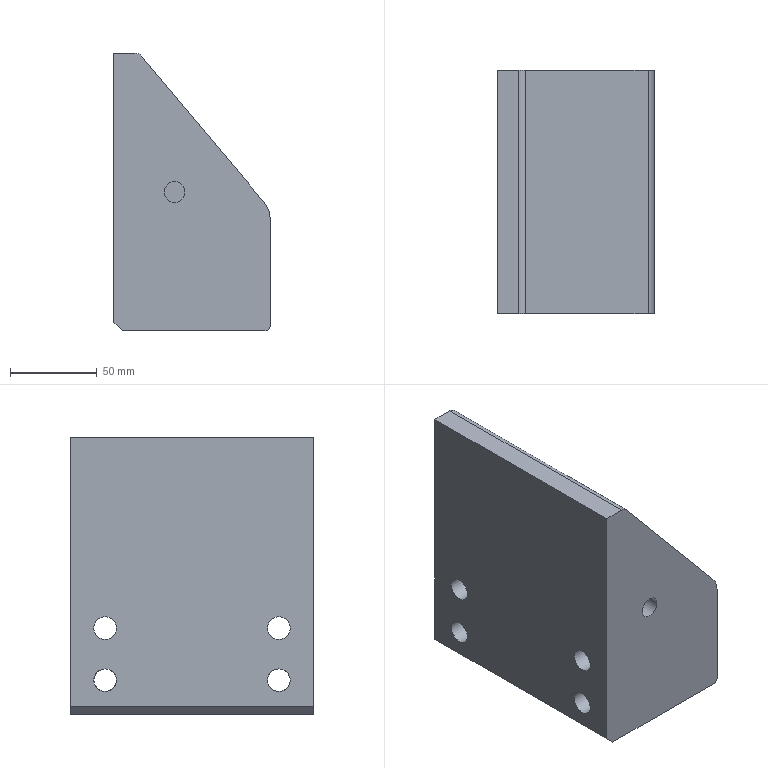Part | NX | features MAIN_BODY 2 | 1 solid | 27 faces | box 90 x 140 x 160 mm | volume 1435895 mm3 | plane 14 | cylinder 13 | commonest cylinder face diameters 13 x4 20 x4 12 x2 6 x1 10 x1 30 x1
STEP:
#1=CARTESIAN_POINT('',(780.,255.,-157.));
#2=VERTEX_POINT('',#1);
#3=CARTESIAN_POINT('',(780.,255.,-95.46));
#4=VERTEX_POINT('',#3);
#5=CARTESIAN_POINT('',(780.,255.,34.907));
#6=DIRECTION('',(0.,0.,1.));
#7=VECTOR('',#6,1000.);
#8=LINE('',#5,#7);
#9=EDGE_CURVE('',#2,#4,#8,.T.);
#10=ORIENTED_EDGE('',*,*,#9,.T.);
#11=CARTESIAN_POINT('',(780.,115.,-95.46));
#12=VERTEX_POINT('',#11);
#13=CARTESIAN_POINT('',(780.,145.,-95.46));
#14=DIRECTION('',(0.,1.,0.));
#15=VECTOR('',#14,1000.);
#16=LINE('',#13,#15);
#17=EDGE_CURVE('',#4,#12,#16,.F.);
#18=ORIENTED_EDGE('',*,*,#17,.T.);
#19=CARTESIAN_POINT('',(780.,115.,-157.));
#20=VERTEX_POINT('',#19);
#21=CARTESIAN_POINT('',(780.,115.,-165.));
#22=DIRECTION('',(0.,0.,-1.));
#23=VECTOR('',#22,1000.);
#24=LINE('',#21,#23);
#25=EDGE_CURVE('',#12,#20,#24,.T.);
#26=ORIENTED_EDGE('',*,*,#25,.T.);
#27=CARTESIAN_POINT('',(780.,350.,-157.));
#28=DIRECTION('',(0.,1.,0.));
#29=VECTOR('',#28,1000.);
#30=LINE('',#27,#29);
#31=EDGE_CURVE('',#20,#2,#30,.T.);
#32=ORIENTED_EDGE('',*,*,#31,.T.);
#33=EDGE_LOOP('',(#10,#18,#26,#32));
#34=FACE_BOUND('',#33,.T.);
#35=CARTESIAN_POINT('',(780.,135.,-100.));
#36=VERTEX_POINT('',#35);
#37=CARTESIAN_POINT('',(780.,135.,-110.));
#38=DIRECTION('',(1.,0.,0.));
#39=DIRECTION('',(0.,0.,1.));
#40=AXIS2_PLACEMENT_3D('',#37,#38,#39);
#41=CIRCLE('',#40,10.);
#42=EDGE_CURVE('',#36,#36,#41,.T.);
#43=ORIENTED_EDGE('',*,*,#42,.F.);
#44=EDGE_LOOP('',(#43));
#45=FACE_BOUND('',#44,.T.);
#46=CARTESIAN_POINT('',(780.,245.,-140.));
#47=VERTEX_POINT('',#46);
#48=CARTESIAN_POINT('',(780.,235.,-140.));
#49=DIRECTION('',(1.,0.,0.));
#50=DIRECTION('',(0.,1.,0.));
#51=AXIS2_PLACEMENT_3D('',#48,#49,#50);
#52=CIRCLE('',#51,10.);
#53=EDGE_CURVE('',#47,#47,#52,.F.);
#54=ORIENTED_EDGE('',*,*,#53,.T.);
#55=EDGE_LOOP('',(#54));
#56=FACE_BOUND('',#55,.T.);
#57=CARTESIAN_POINT('',(780.,235.,-100.));
#58=VERTEX_POINT('',#57);
#59=CARTESIAN_POINT('',(780.,235.,-110.));
#60=DIRECTION('',(1.,0.,0.));
#61=DIRECTION('',(0.,0.,1.));
#62=AXIS2_PLACEMENT_3D('',#59,#60,#61);
#63=CIRCLE('',#62,10.);
#64=EDGE_CURVE('',#58,#58,#63,.T.);
#65=ORIENTED_EDGE('',*,*,#64,.F.);
#66=EDGE_LOOP('',(#65));
#67=FACE_BOUND('',#66,.T.);
#68=CARTESIAN_POINT('',(780.,145.,-140.));
#69=VERTEX_POINT('',#68);
#70=CARTESIAN_POINT('',(780.,135.,-140.));
#71=DIRECTION('',(1.,0.,0.));
#72=DIRECTION('',(0.,1.,0.));
#73=AXIS2_PLACEMENT_3D('',#70,#71,#72);
#74=CIRCLE('',#73,10.);
#75=EDGE_CURVE('',#69,#69,#74,.F.);
#76=ORIENTED_EDGE('',*,*,#75,.T.);
#77=EDGE_LOOP('',(#76));
#78=FACE_BOUND('',#77,.T.);
#79=CARTESIAN_POINT('',(780.,350.,-165.));
#80=DIRECTION('',(1.,0.,0.));
#81=DIRECTION('',(0.,1.,0.));
#82=AXIS2_PLACEMENT_3D('',#79,#80,#81);
#83=PLANE('',#82);
#84=ADVANCED_FACE('',(#34,#45,#56,#67,#78),#83,.T.);
#85=CARTESIAN_POINT('',(725.,255.,-74.));
#86=VERTEX_POINT('',#85);
#87=CARTESIAN_POINT('',(725.,255.,-80.));
#88=DIRECTION('',(0.,-1.,0.));
#89=DIRECTION('',(0.,0.,1.));
#90=AXIS2_PLACEMENT_3D('',#87,#88,#89);
#91=CIRCLE('',#90,6.);
#92=EDGE_CURVE('',#86,#86,#91,.T.);
#93=ORIENTED_EDGE('',*,*,#92,.F.);
#94=EDGE_LOOP('',(#93));
#95=FACE_BOUND('',#94,.T.);
#96=CARTESIAN_POINT('',(725.,225.,-74.));
#97=VERTEX_POINT('',#96);
#98=CARTESIAN_POINT('',(725.,225.,-80.));
#99=DIRECTION('',(0.,-1.,0.));
#100=DIRECTION('',(0.,0.,1.));
#101=AXIS2_PLACEMENT_3D('',#98,#99,#100);
#102=CIRCLE('',#101,6.);
#103=EDGE_CURVE('',#97,#97,#102,.F.);
#104=ORIENTED_EDGE('',*,*,#103,.F.);
#105=EDGE_LOOP('',(#104));
#106=FACE_BOUND('',#105,.T.);
#107=CARTESIAN_POINT('',(725.,320.,-80.));
#108=DIRECTION('',(0.,1.,0.));
#109=DIRECTION('',(0.,0.,-1.));
#110=AXIS2_PLACEMENT_3D('',#107,#108,#109);
#111=CYLINDRICAL_SURFACE('',#110,6.);
#112=ADVANCED_FACE('',(#95,#106),#111,.F.);
#113=CARTESIAN_POINT('',(776.491,115.,-85.818));
#114=VERTEX_POINT('',#113);
#115=CARTESIAN_POINT('',(705.98,115.,-1.786));
#116=VERTEX_POINT('',#115);
#117=CARTESIAN_POINT('',(780.,115.,-90.));
#118=DIRECTION('',(-0.6428,0.,0.766));
#119=VECTOR('',#118,1000.);
#120=LINE('',#117,#119);
#121=EDGE_CURVE('',#114,#116,#120,.T.);
#122=ORIENTED_EDGE('',*,*,#121,.F.);
#123=CARTESIAN_POINT('',(776.491,255.,-85.818));
#124=VERTEX_POINT('',#123);
#125=CARTESIAN_POINT('',(776.491,275.,-85.818));
#126=DIRECTION('',(0.,1.,0.));
#127=VECTOR('',#126,1000.);
#128=LINE('',#125,#127);
#129=EDGE_CURVE('',#114,#124,#128,.T.);
#130=ORIENTED_EDGE('',*,*,#129,.T.);
#131=CARTESIAN_POINT('',(705.98,255.,-1.786));
#132=VERTEX_POINT('',#131);
#133=CARTESIAN_POINT('',(780.,255.,-90.));
#134=DIRECTION('',(-0.6428,0.,0.766));
#135=VECTOR('',#134,1000.);
#136=LINE('',#133,#135);
#137=EDGE_CURVE('',#124,#132,#136,.T.);
#138=ORIENTED_EDGE('',*,*,#137,.T.);
#139=CARTESIAN_POINT('',(705.98,175.,-1.786));
#140=DIRECTION('',(0.,1.,0.));
#141=VECTOR('',#140,1000.);
#142=LINE('',#139,#141);
#143=EDGE_CURVE('',#132,#116,#142,.F.);
#144=ORIENTED_EDGE('',*,*,#143,.T.);
#145=EDGE_LOOP('',(#122,#130,#138,#144));
#146=FACE_BOUND('',#145,.T.);
#147=CARTESIAN_POINT('',(780.,225.,-90.));
#148=DIRECTION('',(-0.766,0.,-0.6428));
#149=DIRECTION('',(0.6428,0.,-0.766));
#150=AXIS2_PLACEMENT_3D('',#147,#148,#149);
#151=PLANE('',#150);
#152=ADVANCED_FACE('',(#146),#151,.F.);
#153=CARTESIAN_POINT('',(690.,235.,-103.5));
#154=VERTEX_POINT('',#153);
#155=CARTESIAN_POINT('',(690.,235.,-110.));
#156=DIRECTION('',(1.,0.,0.));
#157=DIRECTION('',(0.,0.,1.));
#158=AXIS2_PLACEMENT_3D('',#155,#156,#157);
#159=CIRCLE('',#158,6.5);
#160=EDGE_CURVE('',#154,#154,#159,.F.);
#161=ORIENTED_EDGE('',*,*,#160,.T.);
#162=EDGE_LOOP('',(#161));
#163=FACE_BOUND('',#162,.T.);
#164=CARTESIAN_POINT('',(715.,235.,-103.5));
#165=VERTEX_POINT('',#164);
#166=CARTESIAN_POINT('',(715.,235.,-110.));
#167=DIRECTION('',(1.,0.,0.));
#168=DIRECTION('',(0.,0.,1.));
#169=AXIS2_PLACEMENT_3D('',#166,#167,#168);
#170=CIRCLE('',#169,6.5);
#171=EDGE_CURVE('',#165,#165,#170,.T.);
#172=ORIENTED_EDGE('',*,*,#171,.T.);
#173=EDGE_LOOP('',(#172));
#174=FACE_BOUND('',#173,.T.);
#175=CARTESIAN_POINT('',(780.,235.,-110.));
#176=DIRECTION('',(-1.,0.,0.));
#177=DIRECTION('',(0.,0.,-1.));
#178=AXIS2_PLACEMENT_3D('',#175,#176,#177);
#179=CYLINDRICAL_SURFACE('',#178,6.5);
#180=ADVANCED_FACE('',(#163,#174),#179,.F.);
#181=CARTESIAN_POINT('',(690.,135.,-103.5));
#182=VERTEX_POINT('',#181);
#183=CARTESIAN_POINT('',(690.,135.,-110.));
#184=DIRECTION('',(1.,0.,0.));
#185=DIRECTION('',(0.,0.,1.));
#186=AXIS2_PLACEMENT_3D('',#183,#184,#185);
#187=CIRCLE('',#186,6.5);
#188=EDGE_CURVE('',#182,#182,#187,.F.);
#189=ORIENTED_EDGE('',*,*,#188,.T.);
#190=EDGE_LOOP('',(#189));
#191=FACE_BOUND('',#190,.T.);
#192=CARTESIAN_POINT('',(715.,135.,-103.5));
#193=VERTEX_POINT('',#192);
#194=CARTESIAN_POINT('',(715.,135.,-110.));
#195=DIRECTION('',(1.,0.,0.));
#196=DIRECTION('',(0.,0.,1.));
#197=AXIS2_PLACEMENT_3D('',#194,#195,#196);
#198=CIRCLE('',#197,6.5);
#199=EDGE_CURVE('',#193,#193,#198,.T.);
#200=ORIENTED_EDGE('',*,*,#199,.T.);
#201=EDGE_LOOP('',(#200));
#202=FACE_BOUND('',#201,.T.);
#203=CARTESIAN_POINT('',(780.,135.,-110.));
#204=DIRECTION('',(-1.,0.,0.));
#205=DIRECTION('',(0.,0.,-1.));
#206=AXIS2_PLACEMENT_3D('',#203,#204,#205);
#207=CYLINDRICAL_SURFACE('',#206,6.5);
#208=ADVANCED_FACE('',(#191,#202),#207,.F.);
#209=CARTESIAN_POINT('',(690.,135.,-133.5));
#210=VERTEX_POINT('',#209);
#211=CARTESIAN_POINT('',(690.,135.,-140.));
#212=DIRECTION('',(-1.,0.,0.));
#213=DIRECTION('',(0.,0.,1.));
#214=AXIS2_PLACEMENT_3D('',#211,#212,#213);
#215=CIRCLE('',#214,6.5);
#216=EDGE_CURVE('',#210,#210,#215,.T.);
#217=ORIENTED_EDGE('',*,*,#216,.F.);
#218=EDGE_LOOP('',(#217));
#219=FACE_BOUND('',#218,.T.);
#220=CARTESIAN_POINT('',(690.,235.,-133.5));
#221=VERTEX_POINT('',#220);
#222=CARTESIAN_POINT('',(690.,235.,-140.));
#223=DIRECTION('',(-1.,0.,0.));
#224=DIRECTION('',(0.,0.,1.));
#225=AXIS2_PLACEMENT_3D('',#222,#223,#224);
#226=CIRCLE('',#225,6.5);
#227=EDGE_CURVE('',#221,#221,#226,.T.);
#228=ORIENTED_EDGE('',*,*,#227,.F.);
#229=EDGE_LOOP('',(#228));
#230=FACE_BOUND('',#229,.T.);
#231=ORIENTED_EDGE('',*,*,#160,.F.);
#232=EDGE_LOOP('',(#231));
#233=FACE_BOUND('',#232,.T.);
#234=CARTESIAN_POINT('',(690.,255.,-155.));
#235=VERTEX_POINT('',#234);
#236=CARTESIAN_POINT('',(690.,255.,0.));
#237=VERTEX_POINT('',#236);
#238=CARTESIAN_POINT('',(690.,255.,34.907));
#239=DIRECTION('',(0.,0.,1.));
#240=VECTOR('',#239,1000.);
#241=LINE('',#238,#240);
#242=EDGE_CURVE('',#235,#237,#241,.T.);
#243=ORIENTED_EDGE('',*,*,#242,.F.);
#244=CARTESIAN_POINT('',(690.,115.,-155.));
#245=VERTEX_POINT('',#244);
#246=CARTESIAN_POINT('',(690.,175.,-155.));
#247=DIRECTION('',(0.,-1.,0.));
#248=VECTOR('',#247,1000.);
#249=LINE('',#246,#248);
#250=EDGE_CURVE('',#235,#245,#249,.T.);
#251=ORIENTED_EDGE('',*,*,#250,.T.);
#252=CARTESIAN_POINT('',(690.,115.,0.));
#253=VERTEX_POINT('',#252);
#254=CARTESIAN_POINT('',(690.,115.,-165.));
#255=DIRECTION('',(0.,0.,-1.));
#256=VECTOR('',#255,1000.);
#257=LINE('',#254,#256);
#258=EDGE_CURVE('',#253,#245,#257,.T.);
#259=ORIENTED_EDGE('',*,*,#258,.F.);
#260=CARTESIAN_POINT('',(690.,255.,0.));
#261=DIRECTION('',(0.,1.,0.));
#262=VECTOR('',#261,1000.);
#263=LINE('',#260,#262);
#264=EDGE_CURVE('',#253,#237,#263,.T.);
#265=ORIENTED_EDGE('',*,*,#264,.T.);
#266=EDGE_LOOP('',(#243,#251,#259,#265));
#267=FACE_BOUND('',#266,.T.);
#268=ORIENTED_EDGE('',*,*,#188,.F.);
#269=EDGE_LOOP('',(#268));
#270=FACE_BOUND('',#269,.T.);
#271=CARTESIAN_POINT('',(690.,350.,-165.));
#272=DIRECTION('',(1.,0.,0.));
#273=DIRECTION('',(0.,1.,0.));
#274=AXIS2_PLACEMENT_3D('',#271,#272,#273);
#275=PLANE('',#274);
#276=ADVANCED_FACE('',(#219,#230,#233,#267,#270),#275,.F.);
#277=CARTESIAN_POINT('',(702.149,115.,0.));
#278=VERTEX_POINT('',#277);
#279=CARTESIAN_POINT('',(780.078,115.,0.));
#280=DIRECTION('',(-1.,0.,0.));
#281=VECTOR('',#280,1000.);
#282=LINE('',#279,#281);
#283=EDGE_CURVE('',#278,#253,#282,.T.);
#284=ORIENTED_EDGE('',*,*,#283,.F.);
#285=CARTESIAN_POINT('',(702.149,255.,0.));
#286=VERTEX_POINT('',#285);
#287=CARTESIAN_POINT('',(702.149,325.,0.));
#288=DIRECTION('',(0.,1.,0.));
#289=VECTOR('',#288,1000.);
#290=LINE('',#287,#289);
#291=EDGE_CURVE('',#278,#286,#290,.T.);
#292=ORIENTED_EDGE('',*,*,#291,.T.);
#293=CARTESIAN_POINT('',(780.078,255.,0.));
#294=DIRECTION('',(-1.,0.,0.));
#295=VECTOR('',#294,1000.);
#296=LINE('',#293,#295);
#297=EDGE_CURVE('',#286,#237,#296,.T.);
#298=ORIENTED_EDGE('',*,*,#297,.T.);
#299=ORIENTED_EDGE('',*,*,#264,.F.);
#300=EDGE_LOOP('',(#284,#292,#298,#299));
#301=FACE_BOUND('',#300,.T.);
#302=CARTESIAN_POINT('',(400.,255.,0.));
#303=DIRECTION('',(0.,0.,1.));
#304=DIRECTION('',(-1.,0.,0.));
#305=AXIS2_PLACEMENT_3D('',#302,#303,#304);
#306=PLANE('',#305);
#307=ADVANCED_FACE('',(#301),#306,.T.);
#308=CARTESIAN_POINT('',(777.,115.,-160.));
#309=VERTEX_POINT('',#308);
#310=CARTESIAN_POINT('',(695.,115.,-160.));
#311=VERTEX_POINT('',#310);
#312=CARTESIAN_POINT('',(720.,115.,-160.));
#313=DIRECTION('',(-1.,0.,0.));
#314=VECTOR('',#313,1000.);
#315=LINE('',#312,#314);
#316=EDGE_CURVE('',#309,#311,#315,.T.);
#317=ORIENTED_EDGE('',*,*,#316,.T.);
#318=CARTESIAN_POINT('',(695.,255.,-160.));
#319=VERTEX_POINT('',#318);
#320=CARTESIAN_POINT('',(695.,325.,-160.));
#321=DIRECTION('',(0.,1.,0.));
#322=VECTOR('',#321,1000.);
#323=LINE('',#320,#322);
#324=EDGE_CURVE('',#311,#319,#323,.T.);
#325=ORIENTED_EDGE('',*,*,#324,.T.);
#326=CARTESIAN_POINT('',(777.,255.,-160.));
#327=VERTEX_POINT('',#326);
#328=CARTESIAN_POINT('',(780.078,255.,-160.));
#329=DIRECTION('',(1.,0.,0.));
#330=VECTOR('',#329,1000.);
#331=LINE('',#328,#330);
#332=EDGE_CURVE('',#319,#327,#331,.T.);
#333=ORIENTED_EDGE('',*,*,#332,.T.);
#334=CARTESIAN_POINT('',(777.,350.,-160.));
#335=DIRECTION('',(0.,1.,0.));
#336=VECTOR('',#335,1000.);
#337=LINE('',#334,#336);
#338=EDGE_CURVE('',#327,#309,#337,.F.);
#339=ORIENTED_EDGE('',*,*,#338,.T.);
#340=EDGE_LOOP('',(#317,#325,#333,#339));
#341=FACE_BOUND('',#340,.T.);
#342=CARTESIAN_POINT('',(720.,350.,-160.));
#343=DIRECTION('',(0.,0.,-1.));
#344=DIRECTION('',(0.,1.,0.));
#345=AXIS2_PLACEMENT_3D('',#342,#343,#344);
#346=PLANE('',#345);
#347=ADVANCED_FACE('',(#341),#346,.T.);
#348=CARTESIAN_POINT('',(725.,115.,-74.));
#349=VERTEX_POINT('',#348);
#350=CARTESIAN_POINT('',(725.,115.,-80.));
#351=DIRECTION('',(0.,-1.,0.));
#352=DIRECTION('',(0.,0.,1.));
#353=AXIS2_PLACEMENT_3D('',#350,#351,#352);
#354=CIRCLE('',#353,6.);
#355=EDGE_CURVE('',#349,#349,#354,.T.);
#356=ORIENTED_EDGE('',*,*,#355,.F.);
#357=EDGE_LOOP('',(#356));
#358=FACE_BOUND('',#357,.T.);
#359=ORIENTED_EDGE('',*,*,#25,.F.);
#360=CARTESIAN_POINT('',(765.,115.,-95.46));
#361=DIRECTION('',(0.,-1.,0.));
#362=DIRECTION('',(0.,0.,1.));
#363=AXIS2_PLACEMENT_3D('',#360,#361,#362);
#364=CIRCLE('',#363,15.);
#365=EDGE_CURVE('',#12,#114,#364,.T.);
#366=ORIENTED_EDGE('',*,*,#365,.T.);
#367=ORIENTED_EDGE('',*,*,#121,.T.);
#368=CARTESIAN_POINT('',(702.149,115.,-5.));
#369=DIRECTION('',(0.,-1.,0.));
#370=DIRECTION('',(0.,0.,1.));
#371=AXIS2_PLACEMENT_3D('',#368,#369,#370);
#372=CIRCLE('',#371,5.);
#373=EDGE_CURVE('',#116,#278,#372,.T.);
#374=ORIENTED_EDGE('',*,*,#373,.T.);
#375=ORIENTED_EDGE('',*,*,#283,.T.);
#376=ORIENTED_EDGE('',*,*,#258,.T.);
#377=CARTESIAN_POINT('',(632.586,115.,-97.586));
#378=DIRECTION('',(0.7071,0.,-0.7071));
#379=VECTOR('',#378,1000.);
#380=LINE('',#377,#379);
#381=EDGE_CURVE('',#245,#311,#380,.T.);
#382=ORIENTED_EDGE('',*,*,#381,.T.);
#383=ORIENTED_EDGE('',*,*,#316,.F.);
#384=CARTESIAN_POINT('',(777.,115.,-157.));
#385=DIRECTION('',(0.,-1.,0.));
#386=DIRECTION('',(0.,0.,1.));
#387=AXIS2_PLACEMENT_3D('',#384,#385,#386);
#388=CIRCLE('',#387,3.);
#389=EDGE_CURVE('',#309,#20,#388,.T.);
#390=ORIENTED_EDGE('',*,*,#389,.T.);
#391=EDGE_LOOP('',(#359,#366,#367,#374,#375,#376,#382,#383,#390));
#392=FACE_BOUND('',#391,.T.);
#393=CARTESIAN_POINT('',(780.078,115.,34.907));
#394=DIRECTION('',(0.,-1.,0.));
#395=DIRECTION('',(0.,0.,-1.));
#396=AXIS2_PLACEMENT_3D('',#393,#394,#395);
#397=PLANE('',#396);
#398=ADVANCED_FACE('',(#358,#392),#397,.T.);
#399=ORIENTED_EDGE('',*,*,#92,.T.);
#400=EDGE_LOOP('',(#399));
#401=FACE_BOUND('',#400,.T.);
#402=ORIENTED_EDGE('',*,*,#137,.F.);
#403=CARTESIAN_POINT('',(765.,255.,-95.46));
#404=DIRECTION('',(0.,-1.,0.));
#405=DIRECTION('',(0.,0.,1.));
#406=AXIS2_PLACEMENT_3D('',#403,#404,#405);
#407=CIRCLE('',#406,15.);
#408=EDGE_CURVE('',#124,#4,#407,.F.);
#409=ORIENTED_EDGE('',*,*,#408,.T.);
#410=ORIENTED_EDGE('',*,*,#9,.F.);
#411=CARTESIAN_POINT('',(777.,255.,-157.));
#412=DIRECTION('',(0.,-1.,0.));
#413=DIRECTION('',(0.,0.,1.));
#414=AXIS2_PLACEMENT_3D('',#411,#412,#413);
#415=CIRCLE('',#414,3.);
#416=EDGE_CURVE('',#2,#327,#415,.F.);
#417=ORIENTED_EDGE('',*,*,#416,.T.);
#418=ORIENTED_EDGE('',*,*,#332,.F.);
#419=CARTESIAN_POINT('',(695.,255.,-160.));
#420=DIRECTION('',(-0.7071,0.,0.7071));
#421=VECTOR('',#420,1000.);
#422=LINE('',#419,#421);
#423=EDGE_CURVE('',#319,#235,#422,.T.);
#424=ORIENTED_EDGE('',*,*,#423,.T.);
#425=ORIENTED_EDGE('',*,*,#242,.T.);
#426=ORIENTED_EDGE('',*,*,#297,.F.);
#427=CARTESIAN_POINT('',(702.149,255.,-5.));
#428=DIRECTION('',(0.,-1.,0.));
#429=DIRECTION('',(0.,0.,1.));
#430=AXIS2_PLACEMENT_3D('',#427,#428,#429);
#431=CIRCLE('',#430,5.);
#432=EDGE_CURVE('',#286,#132,#431,.F.);
#433=ORIENTED_EDGE('',*,*,#432,.T.);
#434=EDGE_LOOP('',(#402,#409,#410,#417,#418,#424,#425,#426,#433));
#435=FACE_BOUND('',#434,.T.);
#436=CARTESIAN_POINT('',(780.078,255.,34.907));
#437=DIRECTION('',(0.,-1.,0.));
#438=DIRECTION('',(0.,0.,-1.));
#439=AXIS2_PLACEMENT_3D('',#436,#437,#438);
#440=PLANE('',#439);
#441=ADVANCED_FACE('',(#401,#435),#440,.F.);
#442=ORIENTED_EDGE('',*,*,#42,.T.);
#443=EDGE_LOOP('',(#442));
#444=FACE_BOUND('',#443,.T.);
#445=CARTESIAN_POINT('',(715.,135.,-100.));
#446=VERTEX_POINT('',#445);
#447=CARTESIAN_POINT('',(715.,135.,-110.));
#448=DIRECTION('',(1.,0.,0.));
#449=DIRECTION('',(0.,0.,1.));
#450=AXIS2_PLACEMENT_3D('',#447,#448,#449);
#451=CIRCLE('',#450,10.);
#452=EDGE_CURVE('',#446,#446,#451,.T.);
#453=ORIENTED_EDGE('',*,*,#452,.F.);
#454=EDGE_LOOP('',(#453));
#455=FACE_BOUND('',#454,.T.);
#456=CARTESIAN_POINT('',(780.,135.,-110.));
#457=DIRECTION('',(-1.,0.,0.));
#458=DIRECTION('',(0.,0.,-1.));
#459=AXIS2_PLACEMENT_3D('',#456,#457,#458);
#460=CYLINDRICAL_SURFACE('',#459,10.);
#461=ADVANCED_FACE('',(#444,#455),#460,.F.);
#462=ORIENTED_EDGE('',*,*,#199,.F.);
#463=EDGE_LOOP('',(#462));
#464=FACE_BOUND('',#463,.T.);
#465=ORIENTED_EDGE('',*,*,#452,.T.);
#466=EDGE_LOOP('',(#465));
#467=FACE_BOUND('',#466,.T.);
#468=CARTESIAN_POINT('',(715.,245.,-125.));
#469=DIRECTION('',(1.,0.,0.));
#470=DIRECTION('',(0.,0.,1.));
#471=AXIS2_PLACEMENT_3D('',#468,#469,#470);
#472=PLANE('',#471);
#473=ADVANCED_FACE('',(#464,#467),#472,.T.);
#474=ORIENTED_EDGE('',*,*,#64,.T.);
#475=EDGE_LOOP('',(#474));
#476=FACE_BOUND('',#475,.T.);
#477=CARTESIAN_POINT('',(715.,235.,-100.));
#478=VERTEX_POINT('',#477);
#479=CARTESIAN_POINT('',(715.,235.,-110.));
#480=DIRECTION('',(1.,0.,0.));
#481=DIRECTION('',(0.,0.,1.));
#482=AXIS2_PLACEMENT_3D('',#479,#480,#481);
#483=CIRCLE('',#482,10.);
#484=EDGE_CURVE('',#478,#478,#483,.T.);
#485=ORIENTED_EDGE('',*,*,#484,.F.);
#486=EDGE_LOOP('',(#485));
#487=FACE_BOUND('',#486,.T.);
#488=CARTESIAN_POINT('',(780.,235.,-110.));
#489=DIRECTION('',(-1.,0.,0.));
#490=DIRECTION('',(0.,0.,-1.));
#491=AXIS2_PLACEMENT_3D('',#488,#489,#490);
#492=CYLINDRICAL_SURFACE('',#491,10.);
#493=ADVANCED_FACE('',(#476,#487),#492,.F.);
#494=ORIENTED_EDGE('',*,*,#171,.F.);
#495=EDGE_LOOP('',(#494));
#496=FACE_BOUND('',#495,.T.);
#497=ORIENTED_EDGE('',*,*,#484,.T.);
#498=EDGE_LOOP('',(#497));
#499=FACE_BOUND('',#498,.T.);
#500=CARTESIAN_POINT('',(715.,305.,-125.));
#501=DIRECTION('',(1.,0.,0.));
#502=DIRECTION('',(0.,0.,1.));
#503=AXIS2_PLACEMENT_3D('',#500,#501,#502);
#504=PLANE('',#503);
#505=ADVANCED_FACE('',(#496,#499),#504,.T.);
#506=CARTESIAN_POINT('',(725.,145.,-74.));
#507=VERTEX_POINT('',#506);
#508=CARTESIAN_POINT('',(725.,145.,-80.));
#509=DIRECTION('',(0.,-1.,0.));
#510=DIRECTION('',(0.,0.,1.));
#511=AXIS2_PLACEMENT_3D('',#508,#509,#510);
#512=CIRCLE('',#511,6.);
#513=EDGE_CURVE('',#507,#507,#512,.T.);
#514=ORIENTED_EDGE('',*,*,#513,.F.);
#515=EDGE_LOOP('',(#514));
#516=FACE_BOUND('',#515,.T.);
#517=ORIENTED_EDGE('',*,*,#355,.T.);
#518=EDGE_LOOP('',(#517));
#519=FACE_BOUND('',#518,.T.);
#520=CARTESIAN_POINT('',(725.,230.,-80.));
#521=DIRECTION('',(0.,-1.,0.));
#522=DIRECTION('',(0.,0.,-1.));
#523=AXIS2_PLACEMENT_3D('',#520,#521,#522);
#524=CYLINDRICAL_SURFACE('',#523,6.);
#525=ADVANCED_FACE('',(#516,#519),#524,.F.);
#526=ORIENTED_EDGE('',*,*,#103,.T.);
#527=EDGE_LOOP('',(#526));
#528=FACE_BOUND('',#527,.T.);
#529=CARTESIAN_POINT('',(720.,225.,-85.));
#530=DIRECTION('',(0.,-1.,0.));
#531=DIRECTION('',(0.,0.,1.));
#532=AXIS2_PLACEMENT_3D('',#529,#530,#531);
#533=PLANE('',#532);
#534=ADVANCED_FACE('',(#528),#533,.F.);
#535=ORIENTED_EDGE('',*,*,#513,.T.);
#536=EDGE_LOOP('',(#535));
#537=FACE_BOUND('',#536,.T.);
#538=CARTESIAN_POINT('',(720.,145.,-85.));
#539=DIRECTION('',(0.,-1.,0.));
#540=DIRECTION('',(0.,0.,1.));
#541=AXIS2_PLACEMENT_3D('',#538,#539,#540);
#542=PLANE('',#541);
#543=ADVANCED_FACE('',(#537),#542,.T.);
#544=ORIENTED_EDGE('',*,*,#389,.F.);
#545=ORIENTED_EDGE('',*,*,#338,.F.);
#546=ORIENTED_EDGE('',*,*,#416,.F.);
#547=ORIENTED_EDGE('',*,*,#31,.F.);
#548=EDGE_LOOP('',(#544,#545,#546,#547));
#549=FACE_BOUND('',#548,.T.);
#550=CARTESIAN_POINT('',(777.,350.,-157.));
#551=DIRECTION('',(0.,1.,0.));
#552=DIRECTION('',(0.,0.,-1.));
#553=AXIS2_PLACEMENT_3D('',#550,#551,#552);
#554=CYLINDRICAL_SURFACE('',#553,3.);
#555=ADVANCED_FACE('',(#549),#554,.T.);
#556=ORIENTED_EDGE('',*,*,#373,.F.);
#557=ORIENTED_EDGE('',*,*,#143,.F.);
#558=ORIENTED_EDGE('',*,*,#432,.F.);
#559=ORIENTED_EDGE('',*,*,#291,.F.);
#560=EDGE_LOOP('',(#556,#557,#558,#559));
#561=FACE_BOUND('',#560,.T.);
#562=CARTESIAN_POINT('',(702.149,255.,-5.));
#563=DIRECTION('',(0.,-1.,0.));
#564=DIRECTION('',(0.,0.,1.));
#565=AXIS2_PLACEMENT_3D('',#562,#563,#564);
#566=CYLINDRICAL_SURFACE('',#565,5.);
#567=ADVANCED_FACE('',(#561),#566,.T.);
#568=ORIENTED_EDGE('',*,*,#381,.F.);
#569=ORIENTED_EDGE('',*,*,#250,.F.);
#570=ORIENTED_EDGE('',*,*,#423,.F.);
#571=ORIENTED_EDGE('',*,*,#324,.F.);
#572=EDGE_LOOP('',(#568,#569,#570,#571));
#573=FACE_BOUND('',#572,.T.);
#574=CARTESIAN_POINT('',(695.,350.,-160.));
#575=DIRECTION('',(-0.7071,0.,-0.7071));
#576=DIRECTION('',(-0.7071,0.,0.7071));
#577=AXIS2_PLACEMENT_3D('',#574,#575,#576);
#578=PLANE('',#577);
#579=ADVANCED_FACE('',(#573),#578,.T.);
#580=ORIENTED_EDGE('',*,*,#53,.F.);
#581=EDGE_LOOP('',(#580));
#582=FACE_BOUND('',#581,.T.);
#583=CARTESIAN_POINT('',(715.,235.,-130.));
#584=VERTEX_POINT('',#583);
#585=CARTESIAN_POINT('',(715.,235.,-140.));
#586=DIRECTION('',(1.,0.,0.));
#587=DIRECTION('',(0.,0.,1.));
#588=AXIS2_PLACEMENT_3D('',#585,#586,#587);
#589=CIRCLE('',#588,10.);
#590=EDGE_CURVE('',#584,#584,#589,.T.);
#591=ORIENTED_EDGE('',*,*,#590,.F.);
#592=EDGE_LOOP('',(#591));
#593=FACE_BOUND('',#592,.T.);
#594=CARTESIAN_POINT('',(705.,235.,-140.));
#595=DIRECTION('',(1.,0.,0.));
#596=DIRECTION('',(0.,-1.,0.));
#597=AXIS2_PLACEMENT_3D('',#594,#595,#596);
#598=CYLINDRICAL_SURFACE('',#597,10.);
#599=ADVANCED_FACE('',(#582,#593),#598,.F.);
#600=CARTESIAN_POINT('',(715.,241.5,-140.));
#601=VERTEX_POINT('',#600);
#602=CARTESIAN_POINT('',(715.,235.,-140.));
#603=DIRECTION('',(1.,0.,0.));
#604=DIRECTION('',(0.,1.,0.));
#605=AXIS2_PLACEMENT_3D('',#602,#603,#604);
#606=CIRCLE('',#605,6.5);
#607=EDGE_CURVE('',#601,#601,#606,.T.);
#608=ORIENTED_EDGE('',*,*,#607,.F.);
#609=EDGE_LOOP('',(#608));
#610=FACE_BOUND('',#609,.T.);
#611=ORIENTED_EDGE('',*,*,#590,.T.);
#612=EDGE_LOOP('',(#611));
#613=FACE_BOUND('',#612,.T.);
#614=CARTESIAN_POINT('',(715.,305.,-170.));
#615=DIRECTION('',(-1.,0.,0.));
#616=DIRECTION('',(0.,1.,0.));
#617=AXIS2_PLACEMENT_3D('',#614,#615,#616);
#618=PLANE('',#617);
#619=ADVANCED_FACE('',(#610,#613),#618,.F.);
#620=ORIENTED_EDGE('',*,*,#607,.T.);
#621=EDGE_LOOP('',(#620));
#622=FACE_BOUND('',#621,.T.);
#623=ORIENTED_EDGE('',*,*,#227,.T.);
#624=EDGE_LOOP('',(#623));
#625=FACE_BOUND('',#624,.T.);
#626=CARTESIAN_POINT('',(680.,235.,-140.));
#627=DIRECTION('',(1.,0.,0.));
#628=DIRECTION('',(0.,-1.,0.));
#629=AXIS2_PLACEMENT_3D('',#626,#627,#628);
#630=CYLINDRICAL_SURFACE('',#629,6.5);
#631=ADVANCED_FACE('',(#622,#625),#630,.F.);
#632=ORIENTED_EDGE('',*,*,#75,.F.);
#633=EDGE_LOOP('',(#632));
#634=FACE_BOUND('',#633,.T.);
#635=CARTESIAN_POINT('',(715.,135.,-130.));
#636=VERTEX_POINT('',#635);
#637=CARTESIAN_POINT('',(715.,135.,-140.));
#638=DIRECTION('',(1.,0.,0.));
#639=DIRECTION('',(0.,0.,1.));
#640=AXIS2_PLACEMENT_3D('',#637,#638,#639);
#641=CIRCLE('',#640,10.);
#642=EDGE_CURVE('',#636,#636,#641,.T.);
#643=ORIENTED_EDGE('',*,*,#642,.F.);
#644=EDGE_LOOP('',(#643));
#645=FACE_BOUND('',#644,.T.);
#646=CARTESIAN_POINT('',(705.,135.,-140.));
#647=DIRECTION('',(1.,0.,0.));
#648=DIRECTION('',(0.,-1.,0.));
#649=AXIS2_PLACEMENT_3D('',#646,#647,#648);
#650=CYLINDRICAL_SURFACE('',#649,10.);
#651=ADVANCED_FACE('',(#634,#645),#650,.F.);
#652=CARTESIAN_POINT('',(715.,141.5,-140.));
#653=VERTEX_POINT('',#652);
#654=CARTESIAN_POINT('',(715.,135.,-140.));
#655=DIRECTION('',(1.,0.,0.));
#656=DIRECTION('',(0.,1.,0.));
#657=AXIS2_PLACEMENT_3D('',#654,#655,#656);
#658=CIRCLE('',#657,6.5);
#659=EDGE_CURVE('',#653,#653,#658,.T.);
#660=ORIENTED_EDGE('',*,*,#659,.F.);
#661=EDGE_LOOP('',(#660));
#662=FACE_BOUND('',#661,.T.);
#663=ORIENTED_EDGE('',*,*,#642,.T.);
#664=EDGE_LOOP('',(#663));
#665=FACE_BOUND('',#664,.T.);
#666=CARTESIAN_POINT('',(715.,195.,-170.));
#667=DIRECTION('',(-1.,0.,0.));
#668=DIRECTION('',(0.,1.,0.));
#669=AXIS2_PLACEMENT_3D('',#666,#667,#668);
#670=PLANE('',#669);
#671=ADVANCED_FACE('',(#662,#665),#670,.F.);
#672=ORIENTED_EDGE('',*,*,#659,.T.);
#673=EDGE_LOOP('',(#672));
#674=FACE_BOUND('',#673,.T.);
#675=ORIENTED_EDGE('',*,*,#216,.T.);
#676=EDGE_LOOP('',(#675));
#677=FACE_BOUND('',#676,.T.);
#678=CARTESIAN_POINT('',(680.,135.,-140.));
#679=DIRECTION('',(1.,0.,0.));
#680=DIRECTION('',(0.,-1.,0.));
#681=AXIS2_PLACEMENT_3D('',#678,#679,#680);
#682=CYLINDRICAL_SURFACE('',#681,6.5);
#683=ADVANCED_FACE('',(#674,#677),#682,.F.);
#684=ORIENTED_EDGE('',*,*,#365,.F.);
#685=ORIENTED_EDGE('',*,*,#17,.F.);
#686=ORIENTED_EDGE('',*,*,#408,.F.);
#687=ORIENTED_EDGE('',*,*,#129,.F.);
#688=EDGE_LOOP('',(#684,#685,#686,#687));
#689=FACE_BOUND('',#688,.T.);
#690=CARTESIAN_POINT('',(765.,225.,-95.46));
#691=DIRECTION('',(0.,-1.,0.));
#692=DIRECTION('',(0.,0.,1.));
#693=AXIS2_PLACEMENT_3D('',#690,#691,#692);
#694=CYLINDRICAL_SURFACE('',#693,15.);
#695=ADVANCED_FACE('',(#689),#694,.T.);
#696=CLOSED_SHELL('',(#84,#112,#152,#180,#208,#276,#307,#347,#398,#441,#461,#473,#493,#505,#525,#534,#543,#555,#567,#579,#599,#619,#631,#651,#671,#683,#695));
#697=MANIFOLD_SOLID_BREP('',#696);
#698=(LENGTH_UNIT()NAMED_UNIT(*)SI_UNIT(.MILLI.,.METRE.));
#699=UNCERTAINTY_MEASURE_WITH_UNIT(LENGTH_MEASURE(0.00001),#698,'','');
#700=(NAMED_UNIT(*)PLANE_ANGLE_UNIT()SI_UNIT($,.RADIAN.));
#701=(NAMED_UNIT(*)SI_UNIT($,.STERADIAN.)SOLID_ANGLE_UNIT());
#702=(GEOMETRIC_REPRESENTATION_CONTEXT(3)GLOBAL_UNCERTAINTY_ASSIGNED_CONTEXT((#699))GLOBAL_UNIT_ASSIGNED_CONTEXT((#698,#700,#701))REPRESENTATION_CONTEXT('',''));
#703=ADVANCED_BREP_SHAPE_REPRESENTATION('',(#697),#702);